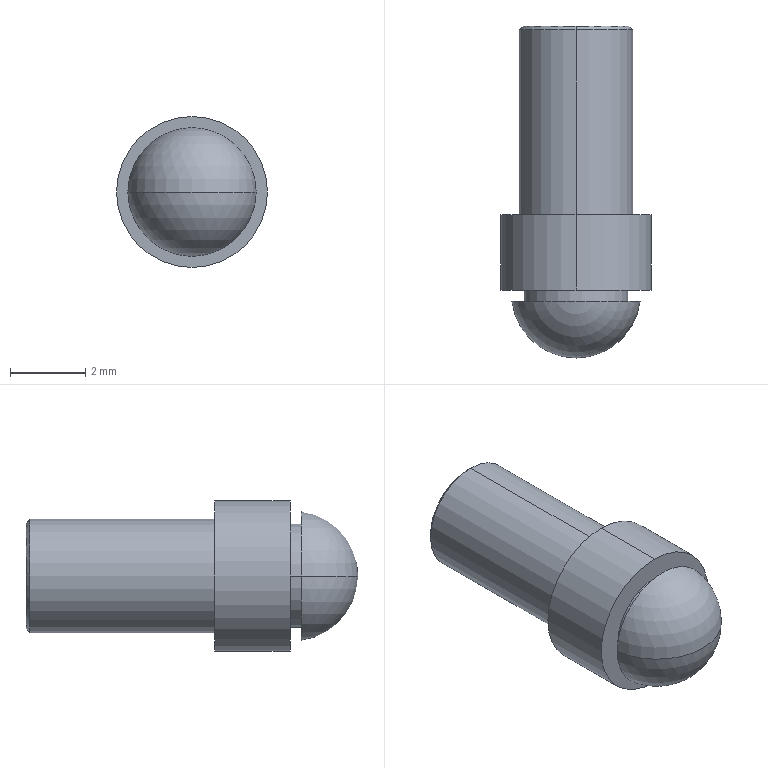Part | SolidWorks | features ICE 2, Chamfer 1, Extrusion 1, Revolution 1 | 1 solid | 21 faces | box 4 x 8.799 x 4 mm | volume 69.832 mm3 | plane 11 | cylinder 6 | cone 2 | sphere 2 | commonest cylinder face diameters 2.753 x2 3 x2 4 x2
STEP:
#1=CARTESIAN_POINT('',(0.,5.,1.4));
#2=VERTEX_POINT('',#1);
#3=CARTESIAN_POINT('',(0.,5.,-1.4));
#4=VERTEX_POINT('',#3);
#5=CARTESIAN_POINT('',(0.,5.,0.));
#6=DIRECTION('',(0.,1.,0.));
#7=DIRECTION('',(0.,0.,1.));
#8=AXIS2_PLACEMENT_3D('',#5,#6,#7);
#9=CIRCLE('',#8,1.4);
#10=EDGE_CURVE('',#2,#4,#9,.T.);
#11=ORIENTED_EDGE('',*,*,#10,.F.);
#12=CARTESIAN_POINT('',(0.,4.9,1.5));
#13=VERTEX_POINT('',#12);
#14=CARTESIAN_POINT('',(0.,5.,1.4));
#15=DIRECTION('',(0.,-0.7071,0.7071));
#16=VECTOR('',#15,1000.);
#17=LINE('',#14,#16);
#18=EDGE_CURVE('',#2,#13,#17,.T.);
#19=ORIENTED_EDGE('',*,*,#18,.T.);
#20=CARTESIAN_POINT('',(0.,4.9,-1.5));
#21=VERTEX_POINT('',#20);
#22=CARTESIAN_POINT('',(0.,4.9,0.));
#23=DIRECTION('',(0.,-1.,0.));
#24=DIRECTION('',(0.,0.,1.));
#25=AXIS2_PLACEMENT_3D('',#22,#23,#24);
#26=CIRCLE('',#25,1.5);
#27=EDGE_CURVE('',#21,#13,#26,.T.);
#28=ORIENTED_EDGE('',*,*,#27,.F.);
#29=CARTESIAN_POINT('',(0.,5.,-1.4));
#30=DIRECTION('',(0.,-0.7071,-0.7071));
#31=VECTOR('',#30,1000.);
#32=LINE('',#29,#31);
#33=EDGE_CURVE('',#4,#21,#32,.T.);
#34=ORIENTED_EDGE('',*,*,#33,.F.);
#35=EDGE_LOOP('',(#11,#19,#28,#34));
#36=FACE_OUTER_BOUND('',#35,.T.);
#37=CARTESIAN_POINT('',(0.,5.,0.));
#38=DIRECTION('',(0.,-1.,0.));
#39=DIRECTION('',(0.,0.,-1.));
#40=AXIS2_PLACEMENT_3D('',#37,#38,#39);
#41=CONICAL_SURFACE('',#40,1.4,0.7854);
#42=ADVANCED_FACE('',(#36),#41,.T.);
#43=CARTESIAN_POINT('',(-1.377,-2.294,0.));
#44=VERTEX_POINT('',#43);
#45=CARTESIAN_POINT('',(1.377,-2.294,0.));
#46=VERTEX_POINT('',#45);
#47=CARTESIAN_POINT('',(0.,-2.294,0.));
#48=DIRECTION('',(0.,1.,0.));
#49=DIRECTION('',(-1.,0.,0.));
#50=AXIS2_PLACEMENT_3D('',#47,#48,#49);
#51=CIRCLE('',#50,1.377);
#52=EDGE_CURVE('',#44,#46,#51,.T.);
#53=ORIENTED_EDGE('',*,*,#52,.T.);
#54=CARTESIAN_POINT('',(1.377,-2.,0.));
#55=VERTEX_POINT('',#54);
#56=CARTESIAN_POINT('',(1.377,-2.,0.));
#57=DIRECTION('',(0.,1.,0.));
#58=VECTOR('',#57,1000.);
#59=LINE('',#56,#58);
#60=EDGE_CURVE('',#46,#55,#59,.T.);
#61=ORIENTED_EDGE('',*,*,#60,.T.);
#62=CARTESIAN_POINT('',(-1.377,-2.,0.));
#63=VERTEX_POINT('',#62);
#64=CARTESIAN_POINT('',(0.,-2.,0.));
#65=DIRECTION('',(0.,1.,0.));
#66=DIRECTION('',(-1.,0.,0.));
#67=AXIS2_PLACEMENT_3D('',#64,#65,#66);
#68=CIRCLE('',#67,1.377);
#69=EDGE_CURVE('',#63,#55,#68,.T.);
#70=ORIENTED_EDGE('',*,*,#69,.F.);
#71=CARTESIAN_POINT('',(-1.377,-2.,0.));
#72=DIRECTION('',(0.,1.,0.));
#73=VECTOR('',#72,1000.);
#74=LINE('',#71,#73);
#75=EDGE_CURVE('',#44,#63,#74,.T.);
#76=ORIENTED_EDGE('',*,*,#75,.F.);
#77=EDGE_LOOP('',(#53,#61,#70,#76));
#78=FACE_OUTER_BOUND('',#77,.T.);
#79=CARTESIAN_POINT('',(0.,-2.,0.));
#80=DIRECTION('',(0.,1.,0.));
#81=DIRECTION('',(-1.,0.,0.));
#82=AXIS2_PLACEMENT_3D('',#79,#80,#81);
#83=CYLINDRICAL_SURFACE('',#82,1.377);
#84=ADVANCED_FACE('',(#78),#83,.T.);
#85=CARTESIAN_POINT('',(0.,-3.799,0.));
#86=VERTEX_POINT('',#85);
#87=CARTESIAN_POINT('',(1.7,-2.294,0.));
#88=VERTEX_POINT('',#87);
#89=CARTESIAN_POINT('',(0.,-2.086,0.));
#90=DIRECTION('',(0.,0.,1.));
#91=DIRECTION('',(1.,0.,0.));
#92=AXIS2_PLACEMENT_3D('',#89,#90,#91);
#93=CIRCLE('',#92,1.713);
#94=EDGE_CURVE('',#86,#88,#93,.T.);
#95=ORIENTED_EDGE('',*,*,#94,.F.);
#96=CARTESIAN_POINT('',(-1.7,-2.294,0.));
#97=VERTEX_POINT('',#96);
#98=CARTESIAN_POINT('',(0.,-2.086,0.));
#99=DIRECTION('',(0.,0.,-1.));
#100=DIRECTION('',(-1.,0.,0.));
#101=AXIS2_PLACEMENT_3D('',#98,#99,#100);
#102=CIRCLE('',#101,1.713);
#103=EDGE_CURVE('',#86,#97,#102,.T.);
#104=ORIENTED_EDGE('',*,*,#103,.T.);
#105=CARTESIAN_POINT('',(0.,-2.294,0.));
#106=DIRECTION('',(0.,1.,0.));
#107=DIRECTION('',(-1.,0.,0.));
#108=AXIS2_PLACEMENT_3D('',#105,#106,#107);
#109=CIRCLE('',#108,1.7);
#110=EDGE_CURVE('',#88,#97,#109,.T.);
#111=ORIENTED_EDGE('',*,*,#110,.F.);
#112=EDGE_LOOP('',(#95,#104,#111));
#113=FACE_OUTER_BOUND('',#112,.T.);
#114=CARTESIAN_POINT('',(0.,-2.086,0.));
#115=DIRECTION('',(0.,0.,-1.));
#116=DIRECTION('',(1.,0.,0.));
#117=AXIS2_PLACEMENT_3D('',#114,#115,#116);
#118=SPHERICAL_SURFACE('',#117,1.713);
#119=ADVANCED_FACE('',(#113),#118,.T.);
#120=CARTESIAN_POINT('',(0.,-2.,-2.));
#121=VERTEX_POINT('',#120);
#122=CARTESIAN_POINT('',(0.,-2.,2.));
#123=VERTEX_POINT('',#122);
#124=CARTESIAN_POINT('',(0.,-2.,0.));
#125=DIRECTION('',(0.,-1.,0.));
#126=DIRECTION('',(0.,0.,-1.));
#127=AXIS2_PLACEMENT_3D('',#124,#125,#126);
#128=CIRCLE('',#127,2.);
#129=EDGE_CURVE('',#121,#123,#128,.T.);
#130=ORIENTED_EDGE('',*,*,#129,.F.);
#131=CARTESIAN_POINT('',(0.,0.,-2.));
#132=VERTEX_POINT('',#131);
#133=CARTESIAN_POINT('',(0.,-2.,-2.));
#134=DIRECTION('',(0.,1.,0.));
#135=VECTOR('',#134,1000.);
#136=LINE('',#133,#135);
#137=EDGE_CURVE('',#121,#132,#136,.T.);
#138=ORIENTED_EDGE('',*,*,#137,.T.);
#139=CARTESIAN_POINT('',(0.,0.,2.));
#140=VERTEX_POINT('',#139);
#141=CARTESIAN_POINT('',(0.,0.,0.));
#142=DIRECTION('',(0.,-1.,0.));
#143=DIRECTION('',(0.,0.,-1.));
#144=AXIS2_PLACEMENT_3D('',#141,#142,#143);
#145=CIRCLE('',#144,2.);
#146=EDGE_CURVE('',#132,#140,#145,.T.);
#147=ORIENTED_EDGE('',*,*,#146,.T.);
#148=CARTESIAN_POINT('',(0.,-2.,2.));
#149=DIRECTION('',(0.,1.,0.));
#150=VECTOR('',#149,1000.);
#151=LINE('',#148,#150);
#152=EDGE_CURVE('',#123,#140,#151,.T.);
#153=ORIENTED_EDGE('',*,*,#152,.F.);
#154=EDGE_LOOP('',(#130,#138,#147,#153));
#155=FACE_OUTER_BOUND('',#154,.T.);
#156=CARTESIAN_POINT('',(0.,-2.,0.));
#157=DIRECTION('',(0.,1.,0.));
#158=DIRECTION('',(0.,0.,1.));
#159=AXIS2_PLACEMENT_3D('',#156,#157,#158);
#160=CYLINDRICAL_SURFACE('',#159,2.);
#161=ADVANCED_FACE('',(#155),#160,.T.);
#162=ORIENTED_EDGE('',*,*,#27,.T.);
#163=CARTESIAN_POINT('',(0.,0.,1.5));
#164=VERTEX_POINT('',#163);
#165=CARTESIAN_POINT('',(0.,5.,1.5));
#166=DIRECTION('',(0.,-1.,0.));
#167=VECTOR('',#166,1000.);
#168=LINE('',#165,#167);
#169=EDGE_CURVE('',#13,#164,#168,.T.);
#170=ORIENTED_EDGE('',*,*,#169,.T.);
#171=CARTESIAN_POINT('',(0.,0.,-1.5));
#172=VERTEX_POINT('',#171);
#173=CARTESIAN_POINT('',(0.,0.,0.));
#174=DIRECTION('',(0.,1.,0.));
#175=DIRECTION('',(0.,0.,1.));
#176=AXIS2_PLACEMENT_3D('',#173,#174,#175);
#177=CIRCLE('',#176,1.5);
#178=EDGE_CURVE('',#164,#172,#177,.T.);
#179=ORIENTED_EDGE('',*,*,#178,.T.);
#180=CARTESIAN_POINT('',(0.,5.,-1.5));
#181=DIRECTION('',(0.,-1.,0.));
#182=VECTOR('',#181,1000.);
#183=LINE('',#180,#182);
#184=EDGE_CURVE('',#21,#172,#183,.T.);
#185=ORIENTED_EDGE('',*,*,#184,.F.);
#186=EDGE_LOOP('',(#162,#170,#179,#185));
#187=FACE_OUTER_BOUND('',#186,.T.);
#188=CARTESIAN_POINT('',(0.,5.,0.));
#189=DIRECTION('',(0.,-1.,0.));
#190=DIRECTION('',(0.,0.,-1.));
#191=AXIS2_PLACEMENT_3D('',#188,#189,#190);
#192=CYLINDRICAL_SURFACE('',#191,1.5);
#193=ADVANCED_FACE('',(#187),#192,.T.);
#194=ORIENTED_EDGE('',*,*,#169,.F.);
#195=CARTESIAN_POINT('',(0.,4.9,0.));
#196=DIRECTION('',(0.,-1.,0.));
#197=DIRECTION('',(0.,0.,1.));
#198=AXIS2_PLACEMENT_3D('',#195,#196,#197);
#199=CIRCLE('',#198,1.5);
#200=EDGE_CURVE('',#13,#21,#199,.T.);
#201=ORIENTED_EDGE('',*,*,#200,.T.);
#202=ORIENTED_EDGE('',*,*,#184,.T.);
#203=CARTESIAN_POINT('',(0.,0.,0.));
#204=DIRECTION('',(0.,1.,0.));
#205=DIRECTION('',(0.,0.,1.));
#206=AXIS2_PLACEMENT_3D('',#203,#204,#205);
#207=CIRCLE('',#206,1.5);
#208=EDGE_CURVE('',#172,#164,#207,.T.);
#209=ORIENTED_EDGE('',*,*,#208,.T.);
#210=EDGE_LOOP('',(#194,#201,#202,#209));
#211=FACE_OUTER_BOUND('',#210,.T.);
#212=CARTESIAN_POINT('',(0.,5.,0.));
#213=DIRECTION('',(0.,-1.,0.));
#214=DIRECTION('',(0.,0.,-1.));
#215=AXIS2_PLACEMENT_3D('',#212,#213,#214);
#216=CYLINDRICAL_SURFACE('',#215,1.5);
#217=ADVANCED_FACE('',(#211),#216,.T.);
#218=CARTESIAN_POINT('',(0.,5.,0.));
#219=DIRECTION('',(0.,1.,0.));
#220=DIRECTION('',(0.,0.,1.));
#221=AXIS2_PLACEMENT_3D('',#218,#219,#220);
#222=CIRCLE('',#221,1.4);
#223=EDGE_CURVE('',#4,#2,#222,.T.);
#224=ORIENTED_EDGE('',*,*,#223,.T.);
#225=ORIENTED_EDGE('',*,*,#10,.T.);
#226=EDGE_LOOP('',(#224,#225));
#227=FACE_OUTER_BOUND('',#226,.T.);
#228=CARTESIAN_POINT('',(0.7449,5.,-0.4301));
#229=VERTEX_POINT('',#228);
#230=CARTESIAN_POINT('',(0.,5.,-0.8602));
#231=VERTEX_POINT('',#230);
#232=CARTESIAN_POINT('',(0.7449,5.,-0.4301));
#233=DIRECTION('',(-0.866,0.,-0.5));
#234=VECTOR('',#233,1000.);
#235=LINE('',#232,#234);
#236=EDGE_CURVE('',#229,#231,#235,.T.);
#237=ORIENTED_EDGE('',*,*,#236,.F.);
#238=CARTESIAN_POINT('',(0.7449,5.,0.4301));
#239=VERTEX_POINT('',#238);
#240=CARTESIAN_POINT('',(0.7449,5.,0.4301));
#241=DIRECTION('',(0.,0.,-1.));
#242=VECTOR('',#241,1000.);
#243=LINE('',#240,#242);
#244=EDGE_CURVE('',#239,#229,#243,.T.);
#245=ORIENTED_EDGE('',*,*,#244,.F.);
#246=CARTESIAN_POINT('',(0.,5.,0.8602));
#247=VERTEX_POINT('',#246);
#248=CARTESIAN_POINT('',(0.,5.,0.8602));
#249=DIRECTION('',(0.866,0.,-0.5));
#250=VECTOR('',#249,1000.);
#251=LINE('',#248,#250);
#252=EDGE_CURVE('',#247,#239,#251,.T.);
#253=ORIENTED_EDGE('',*,*,#252,.F.);
#254=CARTESIAN_POINT('',(-0.7449,5.,0.4301));
#255=VERTEX_POINT('',#254);
#256=CARTESIAN_POINT('',(-0.7449,5.,0.4301));
#257=DIRECTION('',(0.866,0.,0.5));
#258=VECTOR('',#257,1000.);
#259=LINE('',#256,#258);
#260=EDGE_CURVE('',#255,#247,#259,.T.);
#261=ORIENTED_EDGE('',*,*,#260,.F.);
#262=CARTESIAN_POINT('',(-0.7449,5.,-0.4301));
#263=VERTEX_POINT('',#262);
#264=CARTESIAN_POINT('',(-0.7449,5.,-0.4301));
#265=DIRECTION('',(0.,0.,1.));
#266=VECTOR('',#265,1000.);
#267=LINE('',#264,#266);
#268=EDGE_CURVE('',#263,#255,#267,.T.);
#269=ORIENTED_EDGE('',*,*,#268,.F.);
#270=CARTESIAN_POINT('',(0.,5.,-0.8602));
#271=DIRECTION('',(-0.866,0.,0.5));
#272=VECTOR('',#271,1000.);
#273=LINE('',#270,#272);
#274=EDGE_CURVE('',#231,#263,#273,.T.);
#275=ORIENTED_EDGE('',*,*,#274,.F.);
#276=EDGE_LOOP('',(#237,#245,#253,#261,#269,#275));
#277=FACE_BOUND('',#276,.T.);
#278=CARTESIAN_POINT('',(0.,5.,0.));
#279=DIRECTION('',(0.,1.,0.));
#280=DIRECTION('',(0.,0.,1.));
#281=AXIS2_PLACEMENT_3D('',#278,#279,#280);
#282=PLANE('',#281);
#283=ADVANCED_FACE('',(#227,#277),#282,.T.);
#284=ORIENTED_EDGE('',*,*,#137,.F.);
#285=CARTESIAN_POINT('',(0.,-2.,0.));
#286=DIRECTION('',(0.,-1.,0.));
#287=DIRECTION('',(0.,0.,-1.));
#288=AXIS2_PLACEMENT_3D('',#285,#286,#287);
#289=CIRCLE('',#288,2.);
#290=EDGE_CURVE('',#123,#121,#289,.T.);
#291=ORIENTED_EDGE('',*,*,#290,.F.);
#292=ORIENTED_EDGE('',*,*,#152,.T.);
#293=CARTESIAN_POINT('',(0.,0.,0.));
#294=DIRECTION('',(0.,-1.,0.));
#295=DIRECTION('',(0.,0.,-1.));
#296=AXIS2_PLACEMENT_3D('',#293,#294,#295);
#297=CIRCLE('',#296,2.);
#298=EDGE_CURVE('',#140,#132,#297,.T.);
#299=ORIENTED_EDGE('',*,*,#298,.T.);
#300=EDGE_LOOP('',(#284,#291,#292,#299));
#301=FACE_OUTER_BOUND('',#300,.T.);
#302=CARTESIAN_POINT('',(0.,-2.,0.));
#303=DIRECTION('',(0.,1.,0.));
#304=DIRECTION('',(0.,0.,1.));
#305=AXIS2_PLACEMENT_3D('',#302,#303,#304);
#306=CYLINDRICAL_SURFACE('',#305,2.);
#307=ADVANCED_FACE('',(#301),#306,.T.);
#308=ORIENTED_EDGE('',*,*,#69,.T.);
#309=CARTESIAN_POINT('',(0.,-2.,0.));
#310=DIRECTION('',(0.,1.,0.));
#311=DIRECTION('',(-1.,0.,0.));
#312=AXIS2_PLACEMENT_3D('',#309,#310,#311);
#313=CIRCLE('',#312,1.377);
#314=EDGE_CURVE('',#55,#63,#313,.T.);
#315=ORIENTED_EDGE('',*,*,#314,.T.);
#316=EDGE_LOOP('',(#308,#315));
#317=FACE_BOUND('',#316,.T.);
#318=ORIENTED_EDGE('',*,*,#290,.T.);
#319=ORIENTED_EDGE('',*,*,#129,.T.);
#320=EDGE_LOOP('',(#318,#319));
#321=FACE_OUTER_BOUND('',#320,.T.);
#322=CARTESIAN_POINT('',(0.,-2.,0.));
#323=DIRECTION('',(0.,-1.,0.));
#324=DIRECTION('',(0.,0.,-1.));
#325=AXIS2_PLACEMENT_3D('',#322,#323,#324);
#326=PLANE('',#325);
#327=ADVANCED_FACE('',(#317,#321),#326,.T.);
#328=ORIENTED_EDGE('',*,*,#208,.F.);
#329=ORIENTED_EDGE('',*,*,#178,.F.);
#330=EDGE_LOOP('',(#328,#329));
#331=FACE_BOUND('',#330,.T.);
#332=ORIENTED_EDGE('',*,*,#298,.F.);
#333=ORIENTED_EDGE('',*,*,#146,.F.);
#334=EDGE_LOOP('',(#332,#333));
#335=FACE_OUTER_BOUND('',#334,.T.);
#336=CARTESIAN_POINT('',(0.,0.,0.));
#337=DIRECTION('',(0.,-1.,0.));
#338=DIRECTION('',(0.,0.,-1.));
#339=AXIS2_PLACEMENT_3D('',#336,#337,#338);
#340=PLANE('',#339);
#341=ADVANCED_FACE('',(#331,#335),#340,.F.);
#342=ORIENTED_EDGE('',*,*,#103,.F.);
#343=ORIENTED_EDGE('',*,*,#94,.T.);
#344=CARTESIAN_POINT('',(0.,-2.294,0.));
#345=DIRECTION('',(0.,1.,0.));
#346=DIRECTION('',(-1.,0.,0.));
#347=AXIS2_PLACEMENT_3D('',#344,#345,#346);
#348=CIRCLE('',#347,1.7);
#349=EDGE_CURVE('',#97,#88,#348,.T.);
#350=ORIENTED_EDGE('',*,*,#349,.F.);
#351=EDGE_LOOP('',(#342,#343,#350));
#352=FACE_OUTER_BOUND('',#351,.T.);
#353=CARTESIAN_POINT('',(0.,-2.086,0.));
#354=DIRECTION('',(0.,0.,-1.));
#355=DIRECTION('',(1.,0.,0.));
#356=AXIS2_PLACEMENT_3D('',#353,#354,#355);
#357=SPHERICAL_SURFACE('',#356,1.713);
#358=ADVANCED_FACE('',(#352),#357,.T.);
#359=ORIENTED_EDGE('',*,*,#52,.F.);
#360=CARTESIAN_POINT('',(0.,-2.294,0.));
#361=DIRECTION('',(0.,1.,0.));
#362=DIRECTION('',(-1.,0.,0.));
#363=AXIS2_PLACEMENT_3D('',#360,#361,#362);
#364=CIRCLE('',#363,1.377);
#365=EDGE_CURVE('',#46,#44,#364,.T.);
#366=ORIENTED_EDGE('',*,*,#365,.F.);
#367=EDGE_LOOP('',(#359,#366));
#368=FACE_BOUND('',#367,.T.);
#369=ORIENTED_EDGE('',*,*,#110,.T.);
#370=ORIENTED_EDGE('',*,*,#349,.T.);
#371=EDGE_LOOP('',(#369,#370));
#372=FACE_OUTER_BOUND('',#371,.T.);
#373=CARTESIAN_POINT('',(1.377,-2.294,0.));
#374=DIRECTION('',(0.,-1.,0.));
#375=DIRECTION('',(1.,0.,0.));
#376=AXIS2_PLACEMENT_3D('',#373,#374,#375);
#377=PLANE('',#376);
#378=ADVANCED_FACE('',(#368,#372),#377,.F.);
#379=ORIENTED_EDGE('',*,*,#60,.F.);
#380=ORIENTED_EDGE('',*,*,#365,.T.);
#381=ORIENTED_EDGE('',*,*,#75,.T.);
#382=ORIENTED_EDGE('',*,*,#314,.F.);
#383=EDGE_LOOP('',(#379,#380,#381,#382));
#384=FACE_OUTER_BOUND('',#383,.T.);
#385=CARTESIAN_POINT('',(0.,-2.,0.));
#386=DIRECTION('',(0.,1.,0.));
#387=DIRECTION('',(-1.,0.,0.));
#388=AXIS2_PLACEMENT_3D('',#385,#386,#387);
#389=CYLINDRICAL_SURFACE('',#388,1.377);
#390=ADVANCED_FACE('',(#384),#389,.T.);
#391=ORIENTED_EDGE('',*,*,#236,.T.);
#392=CARTESIAN_POINT('',(0.,4.5,-0.8602));
#393=VERTEX_POINT('',#392);
#394=CARTESIAN_POINT('',(0.,4.5,-0.8602));
#395=DIRECTION('',(0.,1.,0.));
#396=VECTOR('',#395,1000.);
#397=LINE('',#394,#396);
#398=EDGE_CURVE('',#393,#231,#397,.T.);
#399=ORIENTED_EDGE('',*,*,#398,.F.);
#400=CARTESIAN_POINT('',(0.7449,4.5,-0.4301));
#401=VERTEX_POINT('',#400);
#402=CARTESIAN_POINT('',(0.7449,4.5,-0.4301));
#403=DIRECTION('',(-0.866,0.,-0.5));
#404=VECTOR('',#403,1000.);
#405=LINE('',#402,#404);
#406=EDGE_CURVE('',#401,#393,#405,.T.);
#407=ORIENTED_EDGE('',*,*,#406,.F.);
#408=CARTESIAN_POINT('',(0.7449,4.5,-0.4301));
#409=DIRECTION('',(0.,1.,0.));
#410=VECTOR('',#409,1000.);
#411=LINE('',#408,#410);
#412=EDGE_CURVE('',#401,#229,#411,.T.);
#413=ORIENTED_EDGE('',*,*,#412,.T.);
#414=EDGE_LOOP('',(#391,#399,#407,#413));
#415=FACE_OUTER_BOUND('',#414,.T.);
#416=CARTESIAN_POINT('',(0.7449,4.5,-0.4301));
#417=DIRECTION('',(0.5,0.,-0.866));
#418=DIRECTION('',(-0.866,0.,-0.5));
#419=AXIS2_PLACEMENT_3D('',#416,#417,#418);
#420=PLANE('',#419);
#421=ADVANCED_FACE('',(#415),#420,.F.);
#422=ORIENTED_EDGE('',*,*,#244,.T.);
#423=ORIENTED_EDGE('',*,*,#412,.F.);
#424=CARTESIAN_POINT('',(0.7449,4.5,0.4301));
#425=VERTEX_POINT('',#424);
#426=CARTESIAN_POINT('',(0.7449,4.5,0.4301));
#427=DIRECTION('',(0.,0.,-1.));
#428=VECTOR('',#427,1000.);
#429=LINE('',#426,#428);
#430=EDGE_CURVE('',#425,#401,#429,.T.);
#431=ORIENTED_EDGE('',*,*,#430,.F.);
#432=CARTESIAN_POINT('',(0.7449,4.5,0.4301));
#433=DIRECTION('',(0.,1.,0.));
#434=VECTOR('',#433,1000.);
#435=LINE('',#432,#434);
#436=EDGE_CURVE('',#425,#239,#435,.T.);
#437=ORIENTED_EDGE('',*,*,#436,.T.);
#438=EDGE_LOOP('',(#422,#423,#431,#437));
#439=FACE_OUTER_BOUND('',#438,.T.);
#440=CARTESIAN_POINT('',(0.7449,4.5,0.4301));
#441=DIRECTION('',(1.,0.,0.));
#442=DIRECTION('',(0.,0.,-1.));
#443=AXIS2_PLACEMENT_3D('',#440,#441,#442);
#444=PLANE('',#443);
#445=ADVANCED_FACE('',(#439),#444,.F.);
#446=ORIENTED_EDGE('',*,*,#252,.T.);
#447=ORIENTED_EDGE('',*,*,#436,.F.);
#448=CARTESIAN_POINT('',(0.,4.5,0.8602));
#449=VERTEX_POINT('',#448);
#450=CARTESIAN_POINT('',(0.,4.5,0.8602));
#451=DIRECTION('',(0.866,0.,-0.5));
#452=VECTOR('',#451,1000.);
#453=LINE('',#450,#452);
#454=EDGE_CURVE('',#449,#425,#453,.T.);
#455=ORIENTED_EDGE('',*,*,#454,.F.);
#456=CARTESIAN_POINT('',(0.,4.5,0.8602));
#457=DIRECTION('',(0.,1.,0.));
#458=VECTOR('',#457,1000.);
#459=LINE('',#456,#458);
#460=EDGE_CURVE('',#449,#247,#459,.T.);
#461=ORIENTED_EDGE('',*,*,#460,.T.);
#462=EDGE_LOOP('',(#446,#447,#455,#461));
#463=FACE_OUTER_BOUND('',#462,.T.);
#464=CARTESIAN_POINT('',(0.,4.5,0.8602));
#465=DIRECTION('',(0.5,0.,0.866));
#466=DIRECTION('',(0.866,0.,-0.5));
#467=AXIS2_PLACEMENT_3D('',#464,#465,#466);
#468=PLANE('',#467);
#469=ADVANCED_FACE('',(#463),#468,.F.);
#470=ORIENTED_EDGE('',*,*,#260,.T.);
#471=ORIENTED_EDGE('',*,*,#460,.F.);
#472=CARTESIAN_POINT('',(-0.7449,4.5,0.4301));
#473=VERTEX_POINT('',#472);
#474=CARTESIAN_POINT('',(-0.7449,4.5,0.4301));
#475=DIRECTION('',(0.866,0.,0.5));
#476=VECTOR('',#475,1000.);
#477=LINE('',#474,#476);
#478=EDGE_CURVE('',#473,#449,#477,.T.);
#479=ORIENTED_EDGE('',*,*,#478,.F.);
#480=CARTESIAN_POINT('',(-0.7449,4.5,0.4301));
#481=DIRECTION('',(0.,1.,0.));
#482=VECTOR('',#481,1000.);
#483=LINE('',#480,#482);
#484=EDGE_CURVE('',#473,#255,#483,.T.);
#485=ORIENTED_EDGE('',*,*,#484,.T.);
#486=EDGE_LOOP('',(#470,#471,#479,#485));
#487=FACE_OUTER_BOUND('',#486,.T.);
#488=CARTESIAN_POINT('',(-0.7449,4.5,0.4301));
#489=DIRECTION('',(-0.5,0.,0.866));
#490=DIRECTION('',(0.866,0.,0.5));
#491=AXIS2_PLACEMENT_3D('',#488,#489,#490);
#492=PLANE('',#491);
#493=ADVANCED_FACE('',(#487),#492,.F.);
#494=ORIENTED_EDGE('',*,*,#268,.T.);
#495=ORIENTED_EDGE('',*,*,#484,.F.);
#496=CARTESIAN_POINT('',(-0.7449,4.5,-0.4301));
#497=VERTEX_POINT('',#496);
#498=CARTESIAN_POINT('',(-0.7449,4.5,-0.4301));
#499=DIRECTION('',(0.,0.,1.));
#500=VECTOR('',#499,1000.);
#501=LINE('',#498,#500);
#502=EDGE_CURVE('',#497,#473,#501,.T.);
#503=ORIENTED_EDGE('',*,*,#502,.F.);
#504=CARTESIAN_POINT('',(-0.7449,4.5,-0.4301));
#505=DIRECTION('',(0.,1.,0.));
#506=VECTOR('',#505,1000.);
#507=LINE('',#504,#506);
#508=EDGE_CURVE('',#497,#263,#507,.T.);
#509=ORIENTED_EDGE('',*,*,#508,.T.);
#510=EDGE_LOOP('',(#494,#495,#503,#509));
#511=FACE_OUTER_BOUND('',#510,.T.);
#512=CARTESIAN_POINT('',(-0.7449,4.5,-0.4301));
#513=DIRECTION('',(-1.,0.,0.));
#514=DIRECTION('',(0.,0.,1.));
#515=AXIS2_PLACEMENT_3D('',#512,#513,#514);
#516=PLANE('',#515);
#517=ADVANCED_FACE('',(#511),#516,.F.);
#518=ORIENTED_EDGE('',*,*,#274,.T.);
#519=ORIENTED_EDGE('',*,*,#508,.F.);
#520=CARTESIAN_POINT('',(0.,4.5,-0.8602));
#521=DIRECTION('',(-0.866,0.,0.5));
#522=VECTOR('',#521,1000.);
#523=LINE('',#520,#522);
#524=EDGE_CURVE('',#393,#497,#523,.T.);
#525=ORIENTED_EDGE('',*,*,#524,.F.);
#526=ORIENTED_EDGE('',*,*,#398,.T.);
#527=EDGE_LOOP('',(#518,#519,#525,#526));
#528=FACE_OUTER_BOUND('',#527,.T.);
#529=CARTESIAN_POINT('',(0.,4.5,-0.8602));
#530=DIRECTION('',(-0.5,0.,-0.866));
#531=DIRECTION('',(-0.866,0.,0.5));
#532=AXIS2_PLACEMENT_3D('',#529,#530,#531);
#533=PLANE('',#532);
#534=ADVANCED_FACE('',(#528),#533,.F.);
#535=ORIENTED_EDGE('',*,*,#406,.T.);
#536=ORIENTED_EDGE('',*,*,#524,.T.);
#537=ORIENTED_EDGE('',*,*,#502,.T.);
#538=ORIENTED_EDGE('',*,*,#478,.T.);
#539=ORIENTED_EDGE('',*,*,#454,.T.);
#540=ORIENTED_EDGE('',*,*,#430,.T.);
#541=EDGE_LOOP('',(#535,#536,#537,#538,#539,#540));
#542=FACE_OUTER_BOUND('',#541,.T.);
#543=CARTESIAN_POINT('',(0.,4.5,0.));
#544=DIRECTION('',(0.,1.,0.));
#545=DIRECTION('',(0.,0.,1.));
#546=AXIS2_PLACEMENT_3D('',#543,#544,#545);
#547=PLANE('',#546);
#548=ADVANCED_FACE('',(#542),#547,.T.);
#549=ORIENTED_EDGE('',*,*,#18,.F.);
#550=ORIENTED_EDGE('',*,*,#223,.F.);
#551=ORIENTED_EDGE('',*,*,#33,.T.);
#552=ORIENTED_EDGE('',*,*,#200,.F.);
#553=EDGE_LOOP('',(#549,#550,#551,#552));
#554=FACE_OUTER_BOUND('',#553,.T.);
#555=CARTESIAN_POINT('',(0.,5.,0.));
#556=DIRECTION('',(0.,-1.,0.));
#557=DIRECTION('',(0.,0.,-1.));
#558=AXIS2_PLACEMENT_3D('',#555,#556,#557);
#559=CONICAL_SURFACE('',#558,1.4,0.7854);
#560=ADVANCED_FACE('',(#554),#559,.T.);
#561=CLOSED_SHELL('',(#42,#84,#119,#161,#193,#217,#283,#307,#327,#341,#358,#378,#390,#421,#445,#469,#493,#517,#534,#548,#560));
#562=MANIFOLD_SOLID_BREP('',#561);
#563=CARTESIAN_POINT('',(0.,0.,0.));
#564=DIRECTION('',(0.,0.,1.));
#565=DIRECTION('',(1.,0.,0.));
#566=AXIS2_PLACEMENT_3D('',#563,#564,#565);
#567=(LENGTH_UNIT()NAMED_UNIT(*)SI_UNIT(.MILLI.,.METRE.));
#568=UNCERTAINTY_MEASURE_WITH_UNIT(LENGTH_MEASURE(0.00001),#567,'','');
#569=(NAMED_UNIT(*)PLANE_ANGLE_UNIT()SI_UNIT($,.RADIAN.));
#570=(NAMED_UNIT(*)SI_UNIT($,.STERADIAN.)SOLID_ANGLE_UNIT());
#571=(GEOMETRIC_REPRESENTATION_CONTEXT(3)GLOBAL_UNCERTAINTY_ASSIGNED_CONTEXT((#568))GLOBAL_UNIT_ASSIGNED_CONTEXT((#567,#569,#570))REPRESENTATION_CONTEXT('',''));
#572=ADVANCED_BREP_SHAPE_REPRESENTATION('',(#562,#566),#571);